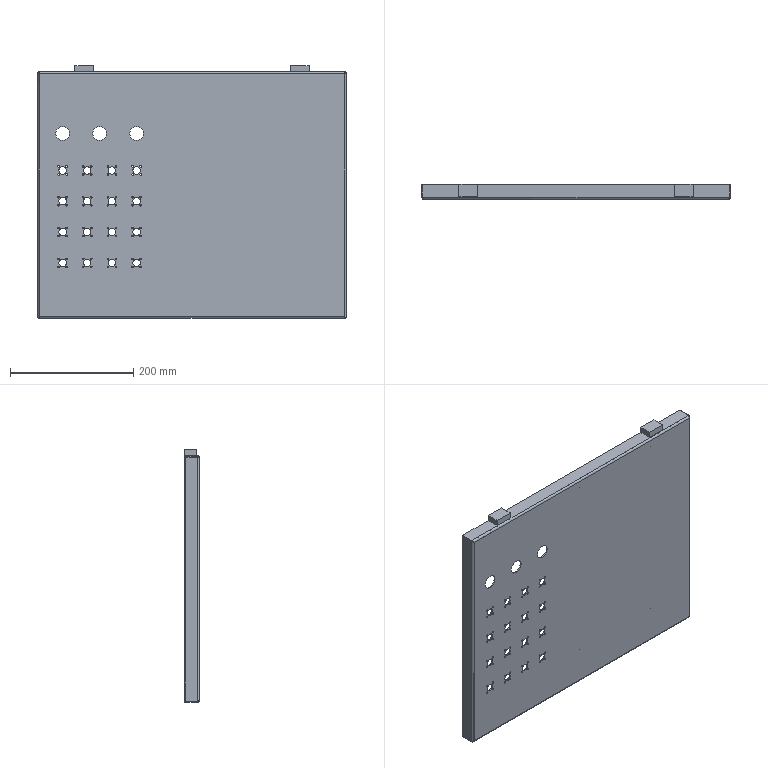Part | STEP file | Station three ctrl box rear cover | 1 solid | 228 faces | box 500 x 24 x 410 mm | volume 510140 mm3 | cylinder 188 | plane 36 | spline 4 | commonest cylinder face diameters 2.5 x128 12 x32 2 x8 4 x8 22.5 x6 6 x4